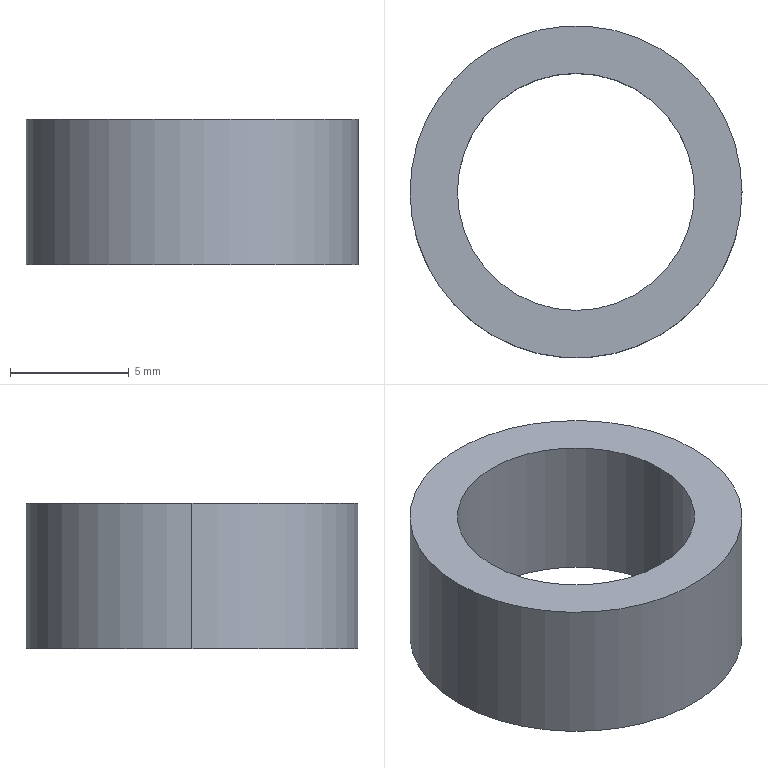Part | SolidWorks | features Extrusion 1 | 1 solid | 6 faces | box 14 x 14 x 6.15 mm | volume 463.699 mm3 | cylinder 4 | plane 2 | commonest cylinder face diameters 10 x2 14 x2
STEP:
#1=CARTESIAN_POINT('',(-5.,0.,6.15));
#2=VERTEX_POINT('',#1);
#3=CARTESIAN_POINT('',(5.,0.,6.15));
#4=VERTEX_POINT('',#3);
#5=CARTESIAN_POINT('',(0.,0.,6.15));
#6=DIRECTION('',(0.,0.,1.));
#7=DIRECTION('',(1.,0.,0.));
#8=AXIS2_PLACEMENT_3D('',#5,#6,#7);
#9=CIRCLE('',#8,5.);
#10=EDGE_CURVE('',#2,#4,#9,.T.);
#11=ORIENTED_EDGE('',*,*,#10,.T.);
#12=CARTESIAN_POINT('',(5.,0.,0.));
#13=VERTEX_POINT('',#12);
#14=CARTESIAN_POINT('',(5.,0.,6.15));
#15=DIRECTION('',(0.,0.,-1.));
#16=VECTOR('',#15,1000.);
#17=LINE('',#14,#16);
#18=EDGE_CURVE('',#4,#13,#17,.T.);
#19=ORIENTED_EDGE('',*,*,#18,.T.);
#20=CARTESIAN_POINT('',(-5.,0.,0.));
#21=VERTEX_POINT('',#20);
#22=CARTESIAN_POINT('',(0.,0.,0.));
#23=DIRECTION('',(0.,0.,1.));
#24=DIRECTION('',(1.,0.,0.));
#25=AXIS2_PLACEMENT_3D('',#22,#23,#24);
#26=CIRCLE('',#25,5.);
#27=EDGE_CURVE('',#21,#13,#26,.T.);
#28=ORIENTED_EDGE('',*,*,#27,.F.);
#29=CARTESIAN_POINT('',(-5.,0.,6.15));
#30=DIRECTION('',(0.,0.,-1.));
#31=VECTOR('',#30,1000.);
#32=LINE('',#29,#31);
#33=EDGE_CURVE('',#2,#21,#32,.T.);
#34=ORIENTED_EDGE('',*,*,#33,.F.);
#35=EDGE_LOOP('',(#11,#19,#28,#34));
#36=FACE_OUTER_BOUND('',#35,.T.);
#37=CARTESIAN_POINT('',(0.,0.,6.15));
#38=DIRECTION('',(0.,0.,-1.));
#39=DIRECTION('',(-1.,0.,0.));
#40=AXIS2_PLACEMENT_3D('',#37,#38,#39);
#41=CYLINDRICAL_SURFACE('',#40,5.);
#42=ADVANCED_FACE('',(#36),#41,.F.);
#43=CARTESIAN_POINT('',(7.,0.,6.15));
#44=VERTEX_POINT('',#43);
#45=CARTESIAN_POINT('',(-7.,0.,6.15));
#46=VERTEX_POINT('',#45);
#47=CARTESIAN_POINT('',(0.,0.,6.15));
#48=DIRECTION('',(0.,0.,1.));
#49=DIRECTION('',(1.,0.,0.));
#50=AXIS2_PLACEMENT_3D('',#47,#48,#49);
#51=CIRCLE('',#50,7.);
#52=EDGE_CURVE('',#44,#46,#51,.T.);
#53=ORIENTED_EDGE('',*,*,#52,.F.);
#54=CARTESIAN_POINT('',(7.,0.,0.));
#55=VERTEX_POINT('',#54);
#56=CARTESIAN_POINT('',(7.,0.,6.15));
#57=DIRECTION('',(0.,0.,-1.));
#58=VECTOR('',#57,1000.);
#59=LINE('',#56,#58);
#60=EDGE_CURVE('',#44,#55,#59,.T.);
#61=ORIENTED_EDGE('',*,*,#60,.T.);
#62=CARTESIAN_POINT('',(-7.,0.,0.));
#63=VERTEX_POINT('',#62);
#64=CARTESIAN_POINT('',(0.,0.,0.));
#65=DIRECTION('',(0.,0.,1.));
#66=DIRECTION('',(1.,0.,0.));
#67=AXIS2_PLACEMENT_3D('',#64,#65,#66);
#68=CIRCLE('',#67,7.);
#69=EDGE_CURVE('',#55,#63,#68,.T.);
#70=ORIENTED_EDGE('',*,*,#69,.T.);
#71=CARTESIAN_POINT('',(-7.,0.,6.15));
#72=DIRECTION('',(0.,0.,-1.));
#73=VECTOR('',#72,1000.);
#74=LINE('',#71,#73);
#75=EDGE_CURVE('',#46,#63,#74,.T.);
#76=ORIENTED_EDGE('',*,*,#75,.F.);
#77=EDGE_LOOP('',(#53,#61,#70,#76));
#78=FACE_OUTER_BOUND('',#77,.T.);
#79=CARTESIAN_POINT('',(0.,0.,6.15));
#80=DIRECTION('',(0.,0.,-1.));
#81=DIRECTION('',(-1.,0.,0.));
#82=AXIS2_PLACEMENT_3D('',#79,#80,#81);
#83=CYLINDRICAL_SURFACE('',#82,7.);
#84=ADVANCED_FACE('',(#78),#83,.T.);
#85=CARTESIAN_POINT('',(0.,0.,6.15));
#86=DIRECTION('',(0.,0.,1.));
#87=DIRECTION('',(1.,0.,0.));
#88=AXIS2_PLACEMENT_3D('',#85,#86,#87);
#89=CIRCLE('',#88,7.);
#90=EDGE_CURVE('',#46,#44,#89,.T.);
#91=ORIENTED_EDGE('',*,*,#90,.T.);
#92=ORIENTED_EDGE('',*,*,#52,.T.);
#93=EDGE_LOOP('',(#91,#92));
#94=FACE_OUTER_BOUND('',#93,.T.);
#95=ORIENTED_EDGE('',*,*,#10,.F.);
#96=CARTESIAN_POINT('',(0.,0.,6.15));
#97=DIRECTION('',(0.,0.,1.));
#98=DIRECTION('',(1.,0.,0.));
#99=AXIS2_PLACEMENT_3D('',#96,#97,#98);
#100=CIRCLE('',#99,5.);
#101=EDGE_CURVE('',#4,#2,#100,.T.);
#102=ORIENTED_EDGE('',*,*,#101,.F.);
#103=EDGE_LOOP('',(#95,#102));
#104=FACE_BOUND('',#103,.T.);
#105=CARTESIAN_POINT('',(0.,0.,6.15));
#106=DIRECTION('',(0.,0.,1.));
#107=DIRECTION('',(1.,0.,0.));
#108=AXIS2_PLACEMENT_3D('',#105,#106,#107);
#109=PLANE('',#108);
#110=ADVANCED_FACE('',(#94,#104),#109,.T.);
#111=CARTESIAN_POINT('',(0.,0.,0.));
#112=DIRECTION('',(0.,0.,1.));
#113=DIRECTION('',(1.,0.,0.));
#114=AXIS2_PLACEMENT_3D('',#111,#112,#113);
#115=CIRCLE('',#114,7.);
#116=EDGE_CURVE('',#63,#55,#115,.T.);
#117=ORIENTED_EDGE('',*,*,#116,.F.);
#118=ORIENTED_EDGE('',*,*,#69,.F.);
#119=EDGE_LOOP('',(#117,#118));
#120=FACE_OUTER_BOUND('',#119,.T.);
#121=ORIENTED_EDGE('',*,*,#27,.T.);
#122=CARTESIAN_POINT('',(0.,0.,0.));
#123=DIRECTION('',(0.,0.,1.));
#124=DIRECTION('',(1.,0.,0.));
#125=AXIS2_PLACEMENT_3D('',#122,#123,#124);
#126=CIRCLE('',#125,5.);
#127=EDGE_CURVE('',#13,#21,#126,.T.);
#128=ORIENTED_EDGE('',*,*,#127,.T.);
#129=EDGE_LOOP('',(#121,#128));
#130=FACE_BOUND('',#129,.T.);
#131=CARTESIAN_POINT('',(0.,0.,0.));
#132=DIRECTION('',(0.,0.,1.));
#133=DIRECTION('',(1.,0.,0.));
#134=AXIS2_PLACEMENT_3D('',#131,#132,#133);
#135=PLANE('',#134);
#136=ADVANCED_FACE('',(#120,#130),#135,.F.);
#137=ORIENTED_EDGE('',*,*,#60,.F.);
#138=ORIENTED_EDGE('',*,*,#90,.F.);
#139=ORIENTED_EDGE('',*,*,#75,.T.);
#140=ORIENTED_EDGE('',*,*,#116,.T.);
#141=EDGE_LOOP('',(#137,#138,#139,#140));
#142=FACE_OUTER_BOUND('',#141,.T.);
#143=CARTESIAN_POINT('',(0.,0.,6.15));
#144=DIRECTION('',(0.,0.,-1.));
#145=DIRECTION('',(-1.,0.,0.));
#146=AXIS2_PLACEMENT_3D('',#143,#144,#145);
#147=CYLINDRICAL_SURFACE('',#146,7.);
#148=ADVANCED_FACE('',(#142),#147,.T.);
#149=ORIENTED_EDGE('',*,*,#18,.F.);
#150=ORIENTED_EDGE('',*,*,#101,.T.);
#151=ORIENTED_EDGE('',*,*,#33,.T.);
#152=ORIENTED_EDGE('',*,*,#127,.F.);
#153=EDGE_LOOP('',(#149,#150,#151,#152));
#154=FACE_OUTER_BOUND('',#153,.T.);
#155=CARTESIAN_POINT('',(0.,0.,6.15));
#156=DIRECTION('',(0.,0.,-1.));
#157=DIRECTION('',(-1.,0.,0.));
#158=AXIS2_PLACEMENT_3D('',#155,#156,#157);
#159=CYLINDRICAL_SURFACE('',#158,5.);
#160=ADVANCED_FACE('',(#154),#159,.F.);
#161=CLOSED_SHELL('',(#42,#84,#110,#136,#148,#160));
#162=MANIFOLD_SOLID_BREP('',#161);
#163=CARTESIAN_POINT('',(0.,0.,0.));
#164=DIRECTION('',(0.,0.,1.));
#165=DIRECTION('',(1.,0.,0.));
#166=AXIS2_PLACEMENT_3D('',#163,#164,#165);
#167=(LENGTH_UNIT()NAMED_UNIT(*)SI_UNIT(.MILLI.,.METRE.));
#168=UNCERTAINTY_MEASURE_WITH_UNIT(LENGTH_MEASURE(0.00001),#167,'','');
#169=(NAMED_UNIT(*)PLANE_ANGLE_UNIT()SI_UNIT($,.RADIAN.));
#170=(NAMED_UNIT(*)SI_UNIT($,.STERADIAN.)SOLID_ANGLE_UNIT());
#171=(GEOMETRIC_REPRESENTATION_CONTEXT(3)GLOBAL_UNCERTAINTY_ASSIGNED_CONTEXT((#168))GLOBAL_UNIT_ASSIGNED_CONTEXT((#167,#169,#170))REPRESENTATION_CONTEXT('',''));
#172=ADVANCED_BREP_SHAPE_REPRESENTATION('',(#162,#166),#171);